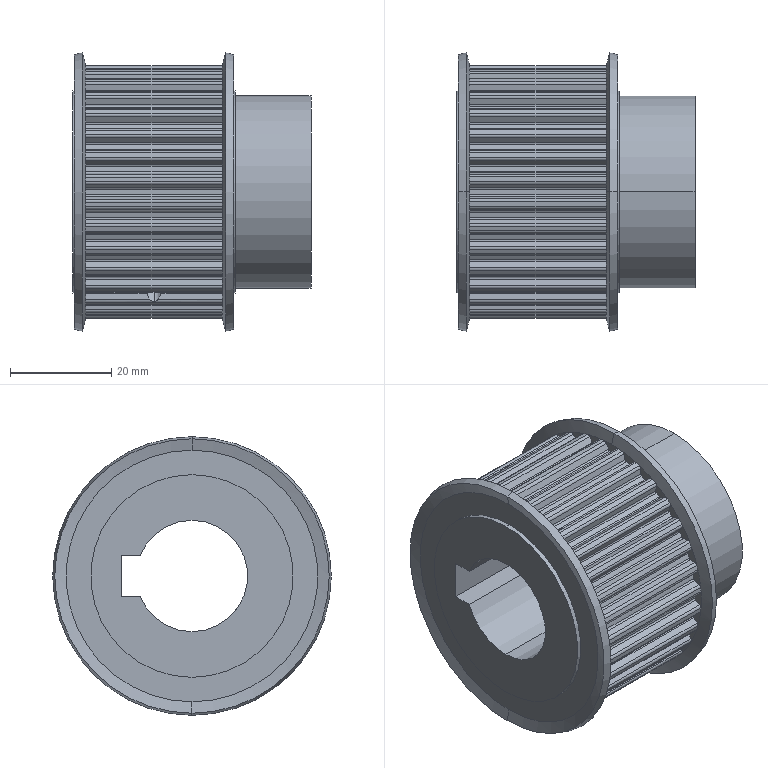Part | STEP file | TTPP32T5250-A-P11_b traction motor pulley SGN-1-10 | 1 solid | 363 faces | box 47 x 55 x 55 mm | volume 57114 mm3 | cylinder 211 | plane 140 | cone 12 | commonest cylinder face diameters 0.8 x68 1.2 x64 46.5 x34 50.1 x32 3.242 x4 40 x4